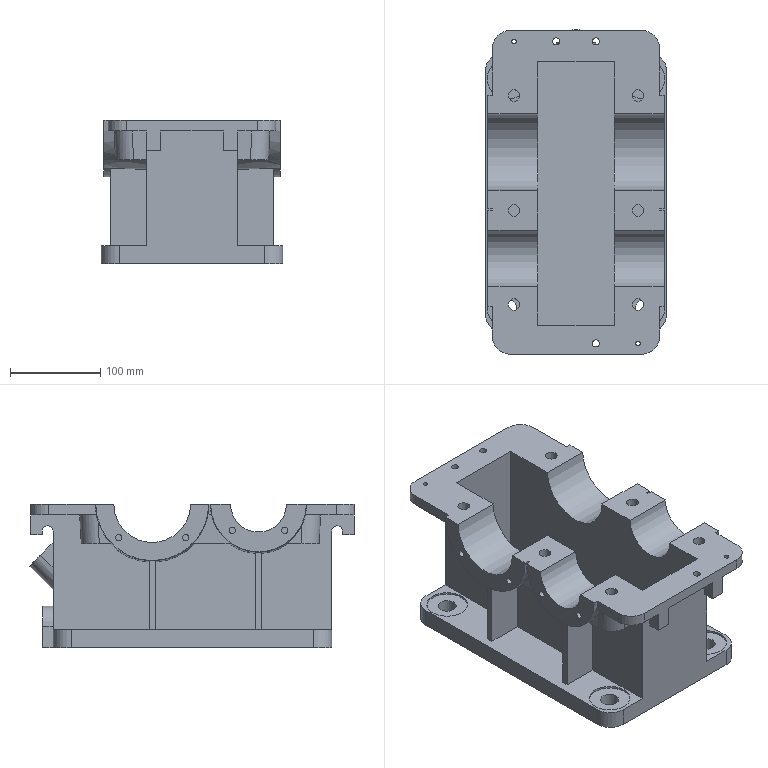Part | NX | features DATUM_CSYS 39, SIMPLE HOLE 38, SKETCH 38, EXTRACT_DATUM_AXIS 32, EXTRACT_FACE 26, HOLE PACKAGE 25, EXTRUDE 22, EXTRACT_DATUM_PLANE 14, Instance Feature 10, DRAFT 8, EXTRACT_STRING 8, BLEND 5, FSET 4, Mirror Feature 4, OFFSET_REGION 3, REPLACE_FACE 3, CPROJ 2, Pattern Feature 2, DATUM_PLANE 1 | 1 solid | 171 faces | box 201 x 359.077 x 159 mm | volume 2835501 mm3 | plane 108 | cylinder 59 | cone 4 | commonest cylinder face diameters 40 x12 7 x8 13 x6 26 x6 20 x5 11.906 x4